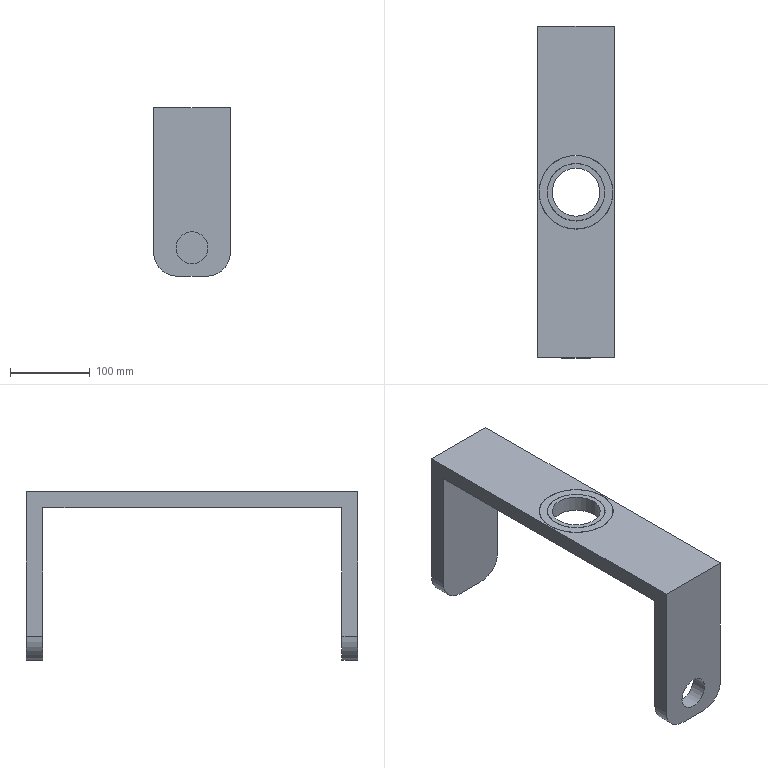Part | NX | features BREP 3 | 3 solids | 24 faces | box 96 x 415 x 211.074 mm | volume 1451349 mm3 | plane 14 | cylinder 10 | commonest cylinder face diameters 60 x5 72 x2 92.501 x2 40 x1
STEP:
#1=CARTESIAN_POINT('',(0.,30.,-10.));
#2=VERTEX_POINT('',#1);
#3=CARTESIAN_POINT('',(0.,0.,-10.));
#4=DIRECTION('',(0.,0.,-1.));
#5=DIRECTION('',(0.,1.,0.));
#6=AXIS2_PLACEMENT_3D('',#3,#4,#5);
#7=CIRCLE('',#6,30.);
#8=EDGE_CURVE('',#2,#2,#7,.T.);
#9=ORIENTED_EDGE('',*,*,#8,.F.);
#10=EDGE_LOOP('',(#9));
#11=FACE_BOUND('',#10,.T.);
#12=CARTESIAN_POINT('',(0.,36.,-10.));
#13=VERTEX_POINT('',#12);
#14=CARTESIAN_POINT('',(0.,0.,-10.));
#15=DIRECTION('',(0.,0.,1.));
#16=DIRECTION('',(0.,1.,0.));
#17=AXIS2_PLACEMENT_3D('',#14,#15,#16);
#18=CIRCLE('',#17,36.);
#19=EDGE_CURVE('',#13,#13,#18,.T.);
#20=ORIENTED_EDGE('',*,*,#19,.F.);
#21=EDGE_LOOP('',(#20));
#22=FACE_BOUND('',#21,.T.);
#23=CARTESIAN_POINT('',(0.,0.,-10.));
#24=DIRECTION('',(0.,0.,-1.));
#25=DIRECTION('',(0.,-1.,0.));
#26=AXIS2_PLACEMENT_3D('',#23,#24,#25);
#27=PLANE('',#26);
#28=ADVANCED_FACE('',(#11,#22),#27,.T.);
#29=CARTESIAN_POINT('',(0.,36.,10.));
#30=VERTEX_POINT('',#29);
#31=CARTESIAN_POINT('',(0.,0.,10.));
#32=DIRECTION('',(0.,0.,1.));
#33=DIRECTION('',(0.,1.,0.));
#34=AXIS2_PLACEMENT_3D('',#31,#32,#33);
#35=CIRCLE('',#34,36.);
#36=EDGE_CURVE('',#30,#30,#35,.T.);
#37=ORIENTED_EDGE('',*,*,#36,.T.);
#38=EDGE_LOOP('',(#37));
#39=FACE_BOUND('',#38,.T.);
#40=CARTESIAN_POINT('',(0.,30.,10.));
#41=VERTEX_POINT('',#40);
#42=CARTESIAN_POINT('',(0.,0.,10.));
#43=DIRECTION('',(0.,0.,-1.));
#44=DIRECTION('',(0.,1.,0.));
#45=AXIS2_PLACEMENT_3D('',#42,#43,#44);
#46=CIRCLE('',#45,30.);
#47=EDGE_CURVE('',#41,#41,#46,.T.);
#48=ORIENTED_EDGE('',*,*,#47,.T.);
#49=EDGE_LOOP('',(#48));
#50=FACE_BOUND('',#49,.T.);
#51=CARTESIAN_POINT('',(0.,0.,10.));
#52=DIRECTION('',(0.,0.,-1.));
#53=DIRECTION('',(0.,-1.,0.));
#54=AXIS2_PLACEMENT_3D('',#51,#52,#53);
#55=PLANE('',#54);
#56=ADVANCED_FACE('',(#39,#50),#55,.F.);
#57=ORIENTED_EDGE('',*,*,#47,.F.);
#58=EDGE_LOOP('',(#57));
#59=FACE_BOUND('',#58,.T.);
#60=ORIENTED_EDGE('',*,*,#8,.T.);
#61=EDGE_LOOP('',(#60));
#62=FACE_BOUND('',#61,.T.);
#63=CARTESIAN_POINT('',(0.,0.,-188.));
#64=DIRECTION('',(0.,0.,1.));
#65=DIRECTION('',(0.,1.,0.));
#66=AXIS2_PLACEMENT_3D('',#63,#64,#65);
#67=CYLINDRICAL_SURFACE('',#66,30.);
#68=ADVANCED_FACE('',(#59,#62),#67,.F.);
#69=ORIENTED_EDGE('',*,*,#36,.F.);
#70=EDGE_LOOP('',(#69));
#71=FACE_BOUND('',#70,.T.);
#72=ORIENTED_EDGE('',*,*,#19,.T.);
#73=EDGE_LOOP('',(#72));
#74=FACE_BOUND('',#73,.T.);
#75=CARTESIAN_POINT('',(0.,0.,-188.));
#76=DIRECTION('',(0.,0.,1.));
#77=DIRECTION('',(0.,1.,0.));
#78=AXIS2_PLACEMENT_3D('',#75,#76,#77);
#79=CYLINDRICAL_SURFACE('',#78,36.);
#80=ADVANCED_FACE('',(#71,#74),#79,.T.);
#81=CLOSED_SHELL('',(#28,#56,#68,#80));
#82=MANIFOLD_SOLID_BREP('',#81);
#83=CARTESIAN_POINT('',(-46.251,0.,-10.));
#84=VERTEX_POINT('',#83);
#85=CARTESIAN_POINT('',(0.,0.,-10.));
#86=DIRECTION('',(0.,0.,1.));
#87=DIRECTION('',(-1.,0.,0.));
#88=AXIS2_PLACEMENT_3D('',#85,#86,#87);
#89=CIRCLE('',#88,46.251);
#90=EDGE_CURVE('',#84,#84,#89,.T.);
#91=ORIENTED_EDGE('',*,*,#90,.T.);
#92=EDGE_LOOP('',(#91));
#93=FACE_BOUND('',#92,.T.);
#94=CARTESIAN_POINT('',(-46.251,0.,10.));
#95=VERTEX_POINT('',#94);
#96=CARTESIAN_POINT('',(0.,0.,10.));
#97=DIRECTION('',(0.,0.,1.));
#98=DIRECTION('',(-1.,0.,0.));
#99=AXIS2_PLACEMENT_3D('',#96,#97,#98);
#100=CIRCLE('',#99,46.251);
#101=EDGE_CURVE('',#95,#95,#100,.T.);
#102=ORIENTED_EDGE('',*,*,#101,.F.);
#103=EDGE_LOOP('',(#102));
#104=FACE_BOUND('',#103,.T.);
#105=CARTESIAN_POINT('',(0.,0.,-10.));
#106=DIRECTION('',(0.,0.,1.));
#107=DIRECTION('',(0.,1.,0.));
#108=AXIS2_PLACEMENT_3D('',#105,#106,#107);
#109=CYLINDRICAL_SURFACE('',#108,46.251);
#110=ADVANCED_FACE('',(#93,#104),#109,.T.);
#111=CARTESIAN_POINT('',(-36.,0.,-10.));
#112=VERTEX_POINT('',#111);
#113=CARTESIAN_POINT('',(0.,0.,-10.));
#114=DIRECTION('',(0.,0.,-1.));
#115=DIRECTION('',(-1.,0.,0.));
#116=AXIS2_PLACEMENT_3D('',#113,#114,#115);
#117=CIRCLE('',#116,36.);
#118=EDGE_CURVE('',#112,#112,#117,.T.);
#119=ORIENTED_EDGE('',*,*,#118,.T.);
#120=EDGE_LOOP('',(#119));
#121=FACE_BOUND('',#120,.T.);
#122=CARTESIAN_POINT('',(-36.,0.,10.));
#123=VERTEX_POINT('',#122);
#124=CARTESIAN_POINT('',(0.,0.,10.));
#125=DIRECTION('',(0.,0.,-1.));
#126=DIRECTION('',(-1.,0.,0.));
#127=AXIS2_PLACEMENT_3D('',#124,#125,#126);
#128=CIRCLE('',#127,36.);
#129=EDGE_CURVE('',#123,#123,#128,.T.);
#130=ORIENTED_EDGE('',*,*,#129,.F.);
#131=EDGE_LOOP('',(#130));
#132=FACE_BOUND('',#131,.T.);
#133=CARTESIAN_POINT('',(0.,0.,-10.));
#134=DIRECTION('',(0.,0.,1.));
#135=DIRECTION('',(0.,1.,0.));
#136=AXIS2_PLACEMENT_3D('',#133,#134,#135);
#137=CYLINDRICAL_SURFACE('',#136,36.);
#138=ADVANCED_FACE('',(#121,#132),#137,.F.);
#139=ORIENTED_EDGE('',*,*,#90,.F.);
#140=EDGE_LOOP('',(#139));
#141=FACE_BOUND('',#140,.T.);
#142=ORIENTED_EDGE('',*,*,#118,.F.);
#143=EDGE_LOOP('',(#142));
#144=FACE_BOUND('',#143,.T.);
#145=CARTESIAN_POINT('',(0.,0.,-10.));
#146=DIRECTION('',(0.,0.,1.));
#147=DIRECTION('',(0.,1.,0.));
#148=AXIS2_PLACEMENT_3D('',#145,#146,#147);
#149=PLANE('',#148);
#150=ADVANCED_FACE('',(#141,#144),#149,.F.);
#151=ORIENTED_EDGE('',*,*,#101,.T.);
#152=EDGE_LOOP('',(#151));
#153=FACE_BOUND('',#152,.T.);
#154=ORIENTED_EDGE('',*,*,#129,.T.);
#155=EDGE_LOOP('',(#154));
#156=FACE_BOUND('',#155,.T.);
#157=CARTESIAN_POINT('',(0.,0.,10.));
#158=DIRECTION('',(0.,0.,1.));
#159=DIRECTION('',(0.,1.,0.));
#160=AXIS2_PLACEMENT_3D('',#157,#158,#159);
#161=PLANE('',#160);
#162=ADVANCED_FACE('',(#153,#156),#161,.T.);
#163=CLOSED_SHELL('',(#110,#138,#150,#162));
#164=MANIFOLD_SOLID_BREP('',#163);
#165=CARTESIAN_POINT('',(0.,46.251,-10.));
#166=VERTEX_POINT('',#165);
#167=CARTESIAN_POINT('',(0.,0.,-10.));
#168=DIRECTION('',(0.,0.,1.));
#169=DIRECTION('',(0.,1.,0.));
#170=AXIS2_PLACEMENT_3D('',#167,#168,#169);
#171=CIRCLE('',#170,46.251);
#172=EDGE_CURVE('',#166,#166,#171,.T.);
#173=ORIENTED_EDGE('',*,*,#172,.T.);
#174=EDGE_LOOP('',(#173));
#175=FACE_BOUND('',#174,.T.);
#176=CARTESIAN_POINT('',(-48.,-187.,-10.));
#177=VERTEX_POINT('',#176);
#178=CARTESIAN_POINT('',(-48.,187.,-10.));
#179=VERTEX_POINT('',#178);
#180=CARTESIAN_POINT('',(-48.,-185.,-10.));
#181=DIRECTION('',(0.,1.,0.));
#182=VECTOR('',#181,1000.);
#183=LINE('',#180,#182);
#184=EDGE_CURVE('',#177,#179,#183,.T.);
#185=ORIENTED_EDGE('',*,*,#184,.T.);
#186=CARTESIAN_POINT('',(48.,187.,-10.));
#187=VERTEX_POINT('',#186);
#188=CARTESIAN_POINT('',(0.,187.,-10.));
#189=DIRECTION('',(1.,0.,0.));
#190=VECTOR('',#189,1000.);
#191=LINE('',#188,#190);
#192=EDGE_CURVE('',#179,#187,#191,.T.);
#193=ORIENTED_EDGE('',*,*,#192,.T.);
#194=CARTESIAN_POINT('',(48.,-187.,-10.));
#195=VERTEX_POINT('',#194);
#196=CARTESIAN_POINT('',(48.,185.,-10.));
#197=DIRECTION('',(0.,-1.,0.));
#198=VECTOR('',#197,1000.);
#199=LINE('',#196,#198);
#200=EDGE_CURVE('',#187,#195,#199,.T.);
#201=ORIENTED_EDGE('',*,*,#200,.T.);
#202=CARTESIAN_POINT('',(0.,-187.,-10.));
#203=DIRECTION('',(1.,0.,0.));
#204=VECTOR('',#203,1000.);
#205=LINE('',#202,#204);
#206=EDGE_CURVE('',#177,#195,#205,.T.);
#207=ORIENTED_EDGE('',*,*,#206,.F.);
#208=EDGE_LOOP('',(#185,#193,#201,#207));
#209=FACE_BOUND('',#208,.T.);
#210=CARTESIAN_POINT('',(0.,0.,-10.));
#211=DIRECTION('',(0.,0.,-1.));
#212=DIRECTION('',(0.,-1.,0.));
#213=AXIS2_PLACEMENT_3D('',#210,#211,#212);
#214=PLANE('',#213);
#215=ADVANCED_FACE('',(#175,#209),#214,.T.);
#216=CARTESIAN_POINT('',(-48.,208.,-171.074));
#217=VERTEX_POINT('',#216);
#218=CARTESIAN_POINT('',(-48.,208.,10.));
#219=VERTEX_POINT('',#218);
#220=CARTESIAN_POINT('',(-48.,208.,-201.074));
#221=DIRECTION('',(0.,0.,1.));
#222=VECTOR('',#221,1000.);
#223=LINE('',#220,#222);
#224=EDGE_CURVE('',#217,#219,#223,.T.);
#225=ORIENTED_EDGE('',*,*,#224,.F.);
#226=CARTESIAN_POINT('',(-48.,187.,-171.074));
#227=VERTEX_POINT('',#226);
#228=CARTESIAN_POINT('',(-48.,-185.,-171.074));
#229=DIRECTION('',(0.,-1.,0.));
#230=VECTOR('',#229,1000.);
#231=LINE('',#228,#230);
#232=EDGE_CURVE('',#217,#227,#231,.T.);
#233=ORIENTED_EDGE('',*,*,#232,.T.);
#234=CARTESIAN_POINT('',(-48.,187.,-201.074));
#235=DIRECTION('',(0.,0.,1.));
#236=VECTOR('',#235,1000.);
#237=LINE('',#234,#236);
#238=EDGE_CURVE('',#227,#179,#237,.T.);
#239=ORIENTED_EDGE('',*,*,#238,.T.);
#240=ORIENTED_EDGE('',*,*,#184,.F.);
#241=CARTESIAN_POINT('',(-48.,-187.,-171.074));
#242=VERTEX_POINT('',#241);
#243=CARTESIAN_POINT('',(-48.,-187.,-201.074));
#244=DIRECTION('',(0.,0.,1.));
#245=VECTOR('',#244,1000.);
#246=LINE('',#243,#245);
#247=EDGE_CURVE('',#242,#177,#246,.T.);
#248=ORIENTED_EDGE('',*,*,#247,.F.);
#249=CARTESIAN_POINT('',(-48.,-207.,-171.074));
#250=VERTEX_POINT('',#249);
#251=CARTESIAN_POINT('',(-48.,-207.,-171.074));
#252=DIRECTION('',(0.,-1.,0.));
#253=VECTOR('',#252,1000.);
#254=LINE('',#251,#253);
#255=EDGE_CURVE('',#242,#250,#254,.T.);
#256=ORIENTED_EDGE('',*,*,#255,.T.);
#257=CARTESIAN_POINT('',(-48.,-207.,10.));
#258=VERTEX_POINT('',#257);
#259=CARTESIAN_POINT('',(-48.,-207.,-201.074));
#260=DIRECTION('',(0.,0.,1.));
#261=VECTOR('',#260,1000.);
#262=LINE('',#259,#261);
#263=EDGE_CURVE('',#250,#258,#262,.T.);
#264=ORIENTED_EDGE('',*,*,#263,.T.);
#265=CARTESIAN_POINT('',(-48.,-185.,10.));
#266=DIRECTION('',(0.,1.,0.));
#267=VECTOR('',#266,1000.);
#268=LINE('',#265,#267);
#269=EDGE_CURVE('',#258,#219,#268,.T.);
#270=ORIENTED_EDGE('',*,*,#269,.T.);
#271=EDGE_LOOP('',(#225,#233,#239,#240,#248,#256,#264,#270));
#272=FACE_BOUND('',#271,.T.);
#273=CARTESIAN_POINT('',(-48.,-185.,-10.));
#274=DIRECTION('',(1.,0.,0.));
#275=DIRECTION('',(0.,-1.,0.));
#276=AXIS2_PLACEMENT_3D('',#273,#274,#275);
#277=PLANE('',#276);
#278=ADVANCED_FACE('',(#272),#277,.F.);
#279=CARTESIAN_POINT('',(48.,187.,-171.074));
#280=VERTEX_POINT('',#279);
#281=CARTESIAN_POINT('',(48.,187.,10.));
#282=DIRECTION('',(0.,0.,-1.));
#283=VECTOR('',#282,1000.);
#284=LINE('',#281,#283);
#285=EDGE_CURVE('',#187,#280,#284,.T.);
#286=ORIENTED_EDGE('',*,*,#285,.T.);
#287=CARTESIAN_POINT('',(48.,208.,-171.074));
#288=VERTEX_POINT('',#287);
#289=CARTESIAN_POINT('',(48.,185.,-171.074));
#290=DIRECTION('',(0.,1.,0.));
#291=VECTOR('',#290,1000.);
#292=LINE('',#289,#291);
#293=EDGE_CURVE('',#280,#288,#292,.T.);
#294=ORIENTED_EDGE('',*,*,#293,.T.);
#295=CARTESIAN_POINT('',(48.,208.,10.));
#296=VERTEX_POINT('',#295);
#297=CARTESIAN_POINT('',(48.,208.,10.));
#298=DIRECTION('',(0.,0.,-1.));
#299=VECTOR('',#298,1000.);
#300=LINE('',#297,#299);
#301=EDGE_CURVE('',#296,#288,#300,.T.);
#302=ORIENTED_EDGE('',*,*,#301,.F.);
#303=CARTESIAN_POINT('',(48.,-207.,10.));
#304=VERTEX_POINT('',#303);
#305=CARTESIAN_POINT('',(48.,185.,10.));
#306=DIRECTION('',(0.,-1.,0.));
#307=VECTOR('',#306,1000.);
#308=LINE('',#305,#307);
#309=EDGE_CURVE('',#296,#304,#308,.T.);
#310=ORIENTED_EDGE('',*,*,#309,.T.);
#311=CARTESIAN_POINT('',(48.,-207.,-171.074));
#312=VERTEX_POINT('',#311);
#313=CARTESIAN_POINT('',(48.,-207.,10.));
#314=DIRECTION('',(0.,0.,-1.));
#315=VECTOR('',#314,1000.);
#316=LINE('',#313,#315);
#317=EDGE_CURVE('',#304,#312,#316,.T.);
#318=ORIENTED_EDGE('',*,*,#317,.T.);
#319=CARTESIAN_POINT('',(48.,-187.,-171.074));
#320=VERTEX_POINT('',#319);
#321=CARTESIAN_POINT('',(48.,-187.,-171.074));
#322=DIRECTION('',(0.,1.,0.));
#323=VECTOR('',#322,1000.);
#324=LINE('',#321,#323);
#325=EDGE_CURVE('',#312,#320,#324,.T.);
#326=ORIENTED_EDGE('',*,*,#325,.T.);
#327=CARTESIAN_POINT('',(48.,-187.,10.));
#328=DIRECTION('',(0.,0.,-1.));
#329=VECTOR('',#328,1000.);
#330=LINE('',#327,#329);
#331=EDGE_CURVE('',#195,#320,#330,.T.);
#332=ORIENTED_EDGE('',*,*,#331,.F.);
#333=ORIENTED_EDGE('',*,*,#200,.F.);
#334=EDGE_LOOP('',(#286,#294,#302,#310,#318,#326,#332,#333));
#335=FACE_BOUND('',#334,.T.);
#336=CARTESIAN_POINT('',(48.,185.,-10.));
#337=DIRECTION('',(-1.,0.,0.));
#338=DIRECTION('',(0.,1.,0.));
#339=AXIS2_PLACEMENT_3D('',#336,#337,#338);
#340=PLANE('',#339);
#341=ADVANCED_FACE('',(#335),#340,.F.);
#342=CARTESIAN_POINT('',(0.,46.251,10.));
#343=VERTEX_POINT('',#342);
#344=CARTESIAN_POINT('',(0.,0.,10.));
#345=DIRECTION('',(0.,0.,1.));
#346=DIRECTION('',(0.,1.,0.));
#347=AXIS2_PLACEMENT_3D('',#344,#345,#346);
#348=CIRCLE('',#347,46.251);
#349=EDGE_CURVE('',#343,#343,#348,.T.);
#350=ORIENTED_EDGE('',*,*,#349,.F.);
#351=EDGE_LOOP('',(#350));
#352=FACE_BOUND('',#351,.T.);
#353=CARTESIAN_POINT('',(-48.,208.,10.));
#354=DIRECTION('',(1.,0.,0.));
#355=VECTOR('',#354,1000.);
#356=LINE('',#353,#355);
#357=EDGE_CURVE('',#219,#296,#356,.T.);
#358=ORIENTED_EDGE('',*,*,#357,.F.);
#359=ORIENTED_EDGE('',*,*,#269,.F.);
#360=CARTESIAN_POINT('',(-48.,-207.,10.));
#361=DIRECTION('',(1.,0.,0.));
#362=VECTOR('',#361,1000.);
#363=LINE('',#360,#362);
#364=EDGE_CURVE('',#258,#304,#363,.T.);
#365=ORIENTED_EDGE('',*,*,#364,.T.);
#366=ORIENTED_EDGE('',*,*,#309,.F.);
#367=EDGE_LOOP('',(#358,#359,#365,#366));
#368=FACE_BOUND('',#367,.T.);
#369=CARTESIAN_POINT('',(0.,0.,10.));
#370=DIRECTION('',(0.,0.,-1.));
#371=DIRECTION('',(0.,-1.,0.));
#372=AXIS2_PLACEMENT_3D('',#369,#370,#371);
#373=PLANE('',#372);
#374=ADVANCED_FACE('',(#352,#368),#373,.F.);
#375=CARTESIAN_POINT('',(18.,-207.,-201.074));
#376=VERTEX_POINT('',#375);
#377=CARTESIAN_POINT('',(-18.,-207.,-201.074));
#378=VERTEX_POINT('',#377);
#379=CARTESIAN_POINT('',(48.,-207.,-201.074));
#380=DIRECTION('',(-1.,0.,0.));
#381=VECTOR('',#380,1000.);
#382=LINE('',#379,#381);
#383=EDGE_CURVE('',#376,#378,#382,.T.);
#384=ORIENTED_EDGE('',*,*,#383,.T.);
#385=CARTESIAN_POINT('',(-18.,-187.,-201.074));
#386=VERTEX_POINT('',#385);
#387=CARTESIAN_POINT('',(-18.,-187.,-201.074));
#388=DIRECTION('',(0.,1.,0.));
#389=VECTOR('',#388,1000.);
#390=LINE('',#387,#389);
#391=EDGE_CURVE('',#378,#386,#390,.T.);
#392=ORIENTED_EDGE('',*,*,#391,.T.);
#393=CARTESIAN_POINT('',(18.,-187.,-201.074));
#394=VERTEX_POINT('',#393);
#395=CARTESIAN_POINT('',(48.,-187.,-201.074));
#396=DIRECTION('',(-1.,0.,0.));
#397=VECTOR('',#396,1000.);
#398=LINE('',#395,#397);
#399=EDGE_CURVE('',#394,#386,#398,.T.);
#400=ORIENTED_EDGE('',*,*,#399,.F.);
#401=CARTESIAN_POINT('',(18.,-207.,-201.074));
#402=DIRECTION('',(0.,-1.,0.));
#403=VECTOR('',#402,1000.);
#404=LINE('',#401,#403);
#405=EDGE_CURVE('',#394,#376,#404,.T.);
#406=ORIENTED_EDGE('',*,*,#405,.T.);
#407=EDGE_LOOP('',(#384,#392,#400,#406));
#408=FACE_BOUND('',#407,.T.);
#409=CARTESIAN_POINT('',(48.,-207.,-201.074));
#410=DIRECTION('',(0.,0.,-1.));
#411=DIRECTION('',(1.,0.,0.));
#412=AXIS2_PLACEMENT_3D('',#409,#410,#411);
#413=PLANE('',#412);
#414=ADVANCED_FACE('',(#408),#413,.T.);
#415=CARTESIAN_POINT('',(-20.,-207.,-165.296));
#416=VERTEX_POINT('',#415);
#417=CARTESIAN_POINT('',(0.,-207.,-165.296));
#418=DIRECTION('',(0.,1.,0.));
#419=DIRECTION('',(-1.,0.,0.));
#420=AXIS2_PLACEMENT_3D('',#417,#418,#419);
#421=CIRCLE('',#420,20.);
#422=EDGE_CURVE('',#416,#416,#421,.T.);
#423=ORIENTED_EDGE('',*,*,#422,.F.);
#424=EDGE_LOOP('',(#423));
#425=FACE_BOUND('',#424,.T.);
#426=CARTESIAN_POINT('',(-20.,-187.,-165.296));
#427=VERTEX_POINT('',#426);
#428=CARTESIAN_POINT('',(0.,-187.,-165.296));
#429=DIRECTION('',(0.,1.,0.));
#430=DIRECTION('',(-1.,0.,0.));
#431=AXIS2_PLACEMENT_3D('',#428,#429,#430);
#432=CIRCLE('',#431,20.);
#433=EDGE_CURVE('',#427,#427,#432,.T.);
#434=ORIENTED_EDGE('',*,*,#433,.T.);
#435=EDGE_LOOP('',(#434));
#436=FACE_BOUND('',#435,.T.);
#437=CARTESIAN_POINT('',(0.,-207.,-165.296));
#438=DIRECTION('',(0.,1.,0.));
#439=DIRECTION('',(0.,0.,-1.));
#440=AXIS2_PLACEMENT_3D('',#437,#438,#439);
#441=CYLINDRICAL_SURFACE('',#440,20.);
#442=ADVANCED_FACE('',(#425,#436),#441,.F.);
#443=ORIENTED_EDGE('',*,*,#263,.F.);
#444=CARTESIAN_POINT('',(-18.,-207.,-171.074));
#445=DIRECTION('',(0.,-1.,0.));
#446=DIRECTION('',(0.,0.,1.));
#447=AXIS2_PLACEMENT_3D('',#444,#445,#446);
#448=CIRCLE('',#447,30.);
#449=EDGE_CURVE('',#250,#378,#448,.T.);
#450=ORIENTED_EDGE('',*,*,#449,.T.);
#451=ORIENTED_EDGE('',*,*,#383,.F.);
#452=CARTESIAN_POINT('',(18.,-207.,-171.074));
#453=DIRECTION('',(0.,-1.,0.));
#454=DIRECTION('',(0.,0.,1.));
#455=AXIS2_PLACEMENT_3D('',#452,#453,#454);
#456=CIRCLE('',#455,30.);
#457=EDGE_CURVE('',#376,#312,#456,.T.);
#458=ORIENTED_EDGE('',*,*,#457,.T.);
#459=ORIENTED_EDGE('',*,*,#317,.F.);
#460=ORIENTED_EDGE('',*,*,#364,.F.);
#461=EDGE_LOOP('',(#443,#450,#451,#458,#459,#460));
#462=FACE_BOUND('',#461,.T.);
#463=ORIENTED_EDGE('',*,*,#422,.T.);
#464=EDGE_LOOP('',(#463));
#465=FACE_BOUND('',#464,.T.);
#466=CARTESIAN_POINT('',(0.,-207.,-165.296));
#467=DIRECTION('',(0.,1.,0.));
#468=DIRECTION('',(0.,0.,-1.));
#469=AXIS2_PLACEMENT_3D('',#466,#467,#468);
#470=PLANE('',#469);
#471=ADVANCED_FACE('',(#462,#465),#470,.F.);
#472=ORIENTED_EDGE('',*,*,#399,.T.);
#473=CARTESIAN_POINT('',(-18.,-187.,-171.074));
#474=DIRECTION('',(0.,1.,0.));
#475=DIRECTION('',(0.,0.,1.));
#476=AXIS2_PLACEMENT_3D('',#473,#474,#475);
#477=CIRCLE('',#476,30.);
#478=EDGE_CURVE('',#386,#242,#477,.T.);
#479=ORIENTED_EDGE('',*,*,#478,.T.);
#480=ORIENTED_EDGE('',*,*,#247,.T.);
#481=ORIENTED_EDGE('',*,*,#206,.T.);
#482=ORIENTED_EDGE('',*,*,#331,.T.);
#483=CARTESIAN_POINT('',(18.,-187.,-171.074));
#484=DIRECTION('',(0.,1.,0.));
#485=DIRECTION('',(0.,0.,1.));
#486=AXIS2_PLACEMENT_3D('',#483,#484,#485);
#487=CIRCLE('',#486,30.);
#488=EDGE_CURVE('',#320,#394,#487,.T.);
#489=ORIENTED_EDGE('',*,*,#488,.T.);
#490=EDGE_LOOP('',(#472,#479,#480,#481,#482,#489));
#491=FACE_BOUND('',#490,.T.);
#492=ORIENTED_EDGE('',*,*,#433,.F.);
#493=EDGE_LOOP('',(#492));
#494=FACE_BOUND('',#493,.T.);
#495=CARTESIAN_POINT('',(0.,-187.,-165.296));
#496=DIRECTION('',(0.,1.,0.));
#497=DIRECTION('',(0.,0.,-1.));
#498=AXIS2_PLACEMENT_3D('',#495,#496,#497);
#499=PLANE('',#498);
#500=ADVANCED_FACE('',(#491,#494),#499,.T.);
#501=CARTESIAN_POINT('',(18.,208.,-201.074));
#502=VERTEX_POINT('',#501);
#503=CARTESIAN_POINT('',(-18.,208.,-201.074));
#504=VERTEX_POINT('',#503);
#505=CARTESIAN_POINT('',(48.,208.,-201.074));
#506=DIRECTION('',(-1.,0.,0.));
#507=VECTOR('',#506,1000.);
#508=LINE('',#505,#507);
#509=EDGE_CURVE('',#502,#504,#508,.T.);
#510=ORIENTED_EDGE('',*,*,#509,.F.);
#511=CARTESIAN_POINT('',(18.,187.,-201.074));
#512=VERTEX_POINT('',#511);
#513=CARTESIAN_POINT('',(18.,208.,-201.074));
#514=DIRECTION('',(0.,-1.,0.));
#515=VECTOR('',#514,1000.);
#516=LINE('',#513,#515);
#517=EDGE_CURVE('',#502,#512,#516,.T.);
#518=ORIENTED_EDGE('',*,*,#517,.T.);
#519=CARTESIAN_POINT('',(-18.,187.,-201.074));
#520=VERTEX_POINT('',#519);
#521=CARTESIAN_POINT('',(48.,187.,-201.074));
#522=DIRECTION('',(-1.,0.,0.));
#523=VECTOR('',#522,1000.);
#524=LINE('',#521,#523);
#525=EDGE_CURVE('',#512,#520,#524,.T.);
#526=ORIENTED_EDGE('',*,*,#525,.T.);
#527=CARTESIAN_POINT('',(-18.,208.,-201.074));
#528=DIRECTION('',(0.,1.,0.));
#529=VECTOR('',#528,1000.);
#530=LINE('',#527,#529);
#531=EDGE_CURVE('',#520,#504,#530,.T.);
#532=ORIENTED_EDGE('',*,*,#531,.T.);
#533=EDGE_LOOP('',(#510,#518,#526,#532));
#534=FACE_BOUND('',#533,.T.);
#535=CARTESIAN_POINT('',(48.,208.,-201.074));
#536=DIRECTION('',(0.,0.,1.));
#537=DIRECTION('',(-1.,0.,0.));
#538=AXIS2_PLACEMENT_3D('',#535,#536,#537);
#539=PLANE('',#538);
#540=ADVANCED_FACE('',(#534),#539,.F.);
#541=ORIENTED_EDGE('',*,*,#301,.T.);
#542=CARTESIAN_POINT('',(18.,208.,-171.074));
#543=DIRECTION('',(0.,1.,0.));
#544=DIRECTION('',(0.,0.,1.));
#545=AXIS2_PLACEMENT_3D('',#542,#543,#544);
#546=CIRCLE('',#545,30.);
#547=EDGE_CURVE('',#288,#502,#546,.T.);
#548=ORIENTED_EDGE('',*,*,#547,.T.);
#549=ORIENTED_EDGE('',*,*,#509,.T.);
#550=CARTESIAN_POINT('',(-18.,208.,-171.074));
#551=DIRECTION('',(0.,1.,0.));
#552=DIRECTION('',(0.,0.,1.));
#553=AXIS2_PLACEMENT_3D('',#550,#551,#552);
#554=CIRCLE('',#553,30.);
#555=EDGE_CURVE('',#504,#217,#554,.T.);
#556=ORIENTED_EDGE('',*,*,#555,.T.);
#557=ORIENTED_EDGE('',*,*,#224,.T.);
#558=ORIENTED_EDGE('',*,*,#357,.T.);
#559=EDGE_LOOP('',(#541,#548,#549,#556,#557,#558));
#560=FACE_BOUND('',#559,.T.);
#561=CARTESIAN_POINT('',(0.,208.,0.));
#562=DIRECTION('',(0.,1.,0.));
#563=DIRECTION('',(0.,0.,-1.));
#564=AXIS2_PLACEMENT_3D('',#561,#562,#563);
#565=PLANE('',#564);
#566=ADVANCED_FACE('',(#560),#565,.T.);
#567=ORIENTED_EDGE('',*,*,#525,.F.);
#568=CARTESIAN_POINT('',(18.,187.,-171.074));
#569=DIRECTION('',(0.,-1.,0.));
#570=DIRECTION('',(0.,0.,1.));
#571=AXIS2_PLACEMENT_3D('',#568,#569,#570);
#572=CIRCLE('',#571,30.);
#573=EDGE_CURVE('',#512,#280,#572,.T.);
#574=ORIENTED_EDGE('',*,*,#573,.T.);
#575=ORIENTED_EDGE('',*,*,#285,.F.);
#576=ORIENTED_EDGE('',*,*,#192,.F.);
#577=ORIENTED_EDGE('',*,*,#238,.F.);
#578=CARTESIAN_POINT('',(-18.,187.,-171.074));
#579=DIRECTION('',(0.,-1.,0.));
#580=DIRECTION('',(0.,0.,1.));
#581=AXIS2_PLACEMENT_3D('',#578,#579,#580);
#582=CIRCLE('',#581,30.);
#583=EDGE_CURVE('',#227,#520,#582,.T.);
#584=ORIENTED_EDGE('',*,*,#583,.T.);
#585=EDGE_LOOP('',(#567,#574,#575,#576,#577,#584));
#586=FACE_BOUND('',#585,.T.);
#587=CARTESIAN_POINT('',(0.,187.,0.));
#588=DIRECTION('',(0.,1.,0.));
#589=DIRECTION('',(0.,0.,-1.));
#590=AXIS2_PLACEMENT_3D('',#587,#588,#589);
#591=PLANE('',#590);
#592=ADVANCED_FACE('',(#586),#591,.F.);
#593=ORIENTED_EDGE('',*,*,#547,.F.);
#594=ORIENTED_EDGE('',*,*,#293,.F.);
#595=ORIENTED_EDGE('',*,*,#573,.F.);
#596=ORIENTED_EDGE('',*,*,#517,.F.);
#597=EDGE_LOOP('',(#593,#594,#595,#596));
#598=FACE_BOUND('',#597,.T.);
#599=CARTESIAN_POINT('',(18.,208.,-171.074));
#600=DIRECTION('',(0.,-1.,0.));
#601=DIRECTION('',(-1.,0.,0.));
#602=AXIS2_PLACEMENT_3D('',#599,#600,#601);
#603=CYLINDRICAL_SURFACE('',#602,30.);
#604=ADVANCED_FACE('',(#598),#603,.T.);
#605=ORIENTED_EDGE('',*,*,#555,.F.);
#606=ORIENTED_EDGE('',*,*,#531,.F.);
#607=ORIENTED_EDGE('',*,*,#583,.F.);
#608=ORIENTED_EDGE('',*,*,#232,.F.);
#609=EDGE_LOOP('',(#605,#606,#607,#608));
#610=FACE_BOUND('',#609,.T.);
#611=CARTESIAN_POINT('',(-18.,-185.,-171.074));
#612=DIRECTION('',(0.,-1.,0.));
#613=DIRECTION('',(-1.,0.,0.));
#614=AXIS2_PLACEMENT_3D('',#611,#612,#613);
#615=CYLINDRICAL_SURFACE('',#614,30.);
#616=ADVANCED_FACE('',(#610),#615,.T.);
#617=ORIENTED_EDGE('',*,*,#449,.F.);
#618=ORIENTED_EDGE('',*,*,#255,.F.);
#619=ORIENTED_EDGE('',*,*,#478,.F.);
#620=ORIENTED_EDGE('',*,*,#391,.F.);
#621=EDGE_LOOP('',(#617,#618,#619,#620));
#622=FACE_BOUND('',#621,.T.);
#623=CARTESIAN_POINT('',(-18.,-207.,-171.074));
#624=DIRECTION('',(0.,-1.,0.));
#625=DIRECTION('',(-1.,0.,0.));
#626=AXIS2_PLACEMENT_3D('',#623,#624,#625);
#627=CYLINDRICAL_SURFACE('',#626,30.);
#628=ADVANCED_FACE('',(#622),#627,.T.);
#629=ORIENTED_EDGE('',*,*,#457,.F.);
#630=ORIENTED_EDGE('',*,*,#405,.F.);
#631=ORIENTED_EDGE('',*,*,#488,.F.);
#632=ORIENTED_EDGE('',*,*,#325,.F.);
#633=EDGE_LOOP('',(#629,#630,#631,#632));
#634=FACE_BOUND('',#633,.T.);
#635=CARTESIAN_POINT('',(18.,185.,-171.074));
#636=DIRECTION('',(0.,-1.,0.));
#637=DIRECTION('',(-1.,0.,0.));
#638=AXIS2_PLACEMENT_3D('',#635,#636,#637);
#639=CYLINDRICAL_SURFACE('',#638,30.);
#640=ADVANCED_FACE('',(#634),#639,.T.);
#641=ORIENTED_EDGE('',*,*,#172,.F.);
#642=EDGE_LOOP('',(#641));
#643=FACE_BOUND('',#642,.T.);
#644=ORIENTED_EDGE('',*,*,#349,.T.);
#645=EDGE_LOOP('',(#644));
#646=FACE_BOUND('',#645,.T.);
#647=CARTESIAN_POINT('',(0.,0.,-70.));
#648=DIRECTION('',(0.,0.,1.));
#649=DIRECTION('',(0.,1.,0.));
#650=AXIS2_PLACEMENT_3D('',#647,#648,#649);
#651=CYLINDRICAL_SURFACE('',#650,46.251);
#652=ADVANCED_FACE('',(#643,#646),#651,.F.);
#653=CLOSED_SHELL('',(#215,#278,#341,#374,#414,#442,#471,#500,#540,#566,#592,#604,#616,#628,#640,#652));
#654=MANIFOLD_SOLID_BREP('',#653);
#655=(LENGTH_UNIT()NAMED_UNIT(*)SI_UNIT(.MILLI.,.METRE.));
#656=UNCERTAINTY_MEASURE_WITH_UNIT(LENGTH_MEASURE(0.00001),#655,'','');
#657=(NAMED_UNIT(*)PLANE_ANGLE_UNIT()SI_UNIT($,.RADIAN.));
#658=(NAMED_UNIT(*)SI_UNIT($,.STERADIAN.)SOLID_ANGLE_UNIT());
#659=(GEOMETRIC_REPRESENTATION_CONTEXT(3)GLOBAL_UNCERTAINTY_ASSIGNED_CONTEXT((#656))GLOBAL_UNIT_ASSIGNED_CONTEXT((#655,#657,#658))REPRESENTATION_CONTEXT('',''));
#660=ADVANCED_BREP_SHAPE_REPRESENTATION('',(#82,#164,#654),#659);